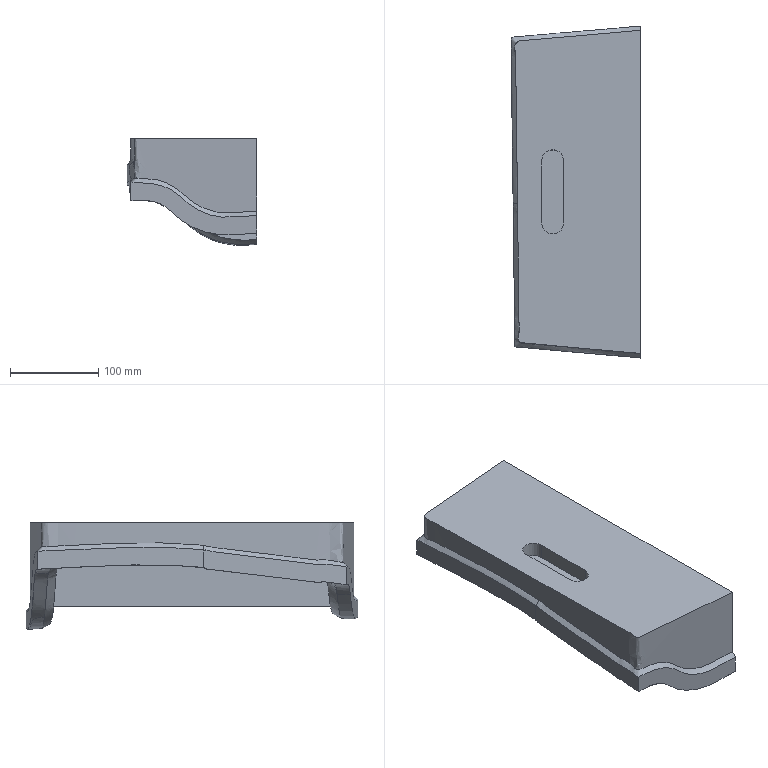Part | NX | features solid 2 | 1 solid | 64 faces | box 147.3 x 376.2 x 120.989 mm | volume 2404277 mm3 | spline 38 | plane 18 | cylinder 8 | commonest cylinder face diameters 30 x5 25 x2 10.05 x1